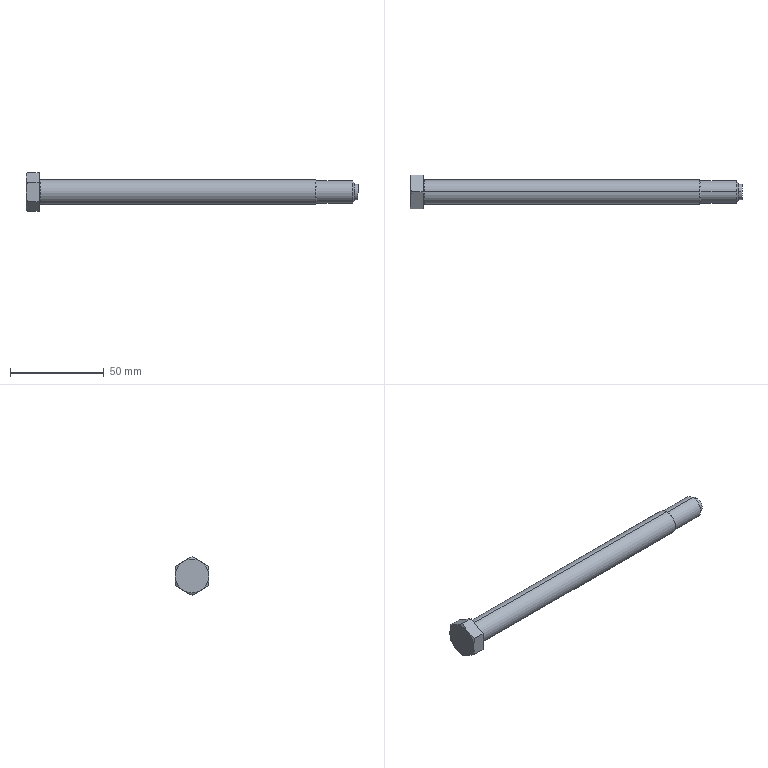Part | SolidWorks | features RevCut 2, Chamfer 1, Extrusion 1, Fillet 1, LPattern 1, MoveCopyBody 1, Revolution 1 | 1 solid | 29 faces | box 177 x 18 x 20.785 mm | volume 23953 mm3 | cone 11 | plane 10 | cylinder 6 | torus 2 | commonest cylinder face diameters 8.5 x2 12 x2 13 x2
STEP:
#1=CARTESIAN_POINT('',(-155.4,0.,169.5));
#2=VERTEX_POINT('',#1);
#3=CARTESIAN_POINT('',(-155.4,0.,156.5));
#4=VERTEX_POINT('',#3);
#5=CARTESIAN_POINT('',(-155.4,0.,163.));
#6=DIRECTION('',(1.,0.,0.));
#7=DIRECTION('',(0.,0.,-1.));
#8=AXIS2_PLACEMENT_3D('',#5,#6,#7);
#9=CIRCLE('',#8,6.5);
#10=EDGE_CURVE('',#2,#4,#9,.T.);
#11=ORIENTED_EDGE('',*,*,#10,.F.);
#12=CARTESIAN_POINT('',(-156.,0.,170.1));
#13=VERTEX_POINT('',#12);
#14=CARTESIAN_POINT('',(-155.4,0.,170.1));
#15=DIRECTION('',(0.,1.,0.));
#16=DIRECTION('',(0.,0.,1.));
#17=AXIS2_PLACEMENT_3D('',#14,#15,#16);
#18=CIRCLE('',#17,0.6);
#19=EDGE_CURVE('',#2,#13,#18,.T.);
#20=ORIENTED_EDGE('',*,*,#19,.T.);
#21=CARTESIAN_POINT('',(-156.,0.,155.9));
#22=VERTEX_POINT('',#21);
#23=CARTESIAN_POINT('',(-156.,0.,163.));
#24=DIRECTION('',(-1.,0.,0.));
#25=DIRECTION('',(0.,0.,-1.));
#26=AXIS2_PLACEMENT_3D('',#23,#24,#25);
#27=CIRCLE('',#26,7.1);
#28=EDGE_CURVE('',#22,#13,#27,.T.);
#29=ORIENTED_EDGE('',*,*,#28,.F.);
#30=CARTESIAN_POINT('',(-155.4,0.,155.9));
#31=DIRECTION('',(0.,-1.,0.));
#32=DIRECTION('',(0.,0.,-1.));
#33=AXIS2_PLACEMENT_3D('',#30,#31,#32);
#34=CIRCLE('',#33,0.6);
#35=EDGE_CURVE('',#4,#22,#34,.T.);
#36=ORIENTED_EDGE('',*,*,#35,.F.);
#37=EDGE_LOOP('',(#11,#20,#29,#36));
#38=FACE_OUTER_BOUND('',#37,.T.);
#39=CARTESIAN_POINT('',(-155.4,0.,163.));
#40=DIRECTION('',(1.,0.,0.));
#41=DIRECTION('',(0.,0.,-1.));
#42=AXIS2_PLACEMENT_3D('',#39,#40,#41);
#43=TOROIDAL_SURFACE('',#42,7.1,0.6);
#44=ADVANCED_FACE('',(#38),#43,.F.);
#45=CARTESIAN_POINT('',(-8.,0.,169.));
#46=VERTEX_POINT('',#45);
#47=CARTESIAN_POINT('',(-8.,0.,157.));
#48=VERTEX_POINT('',#47);
#49=CARTESIAN_POINT('',(-8.,0.,163.));
#50=DIRECTION('',(-1.,0.,0.));
#51=DIRECTION('',(0.,0.,1.));
#52=AXIS2_PLACEMENT_3D('',#49,#50,#51);
#53=CIRCLE('',#52,6.);
#54=EDGE_CURVE('',#46,#48,#53,.T.);
#55=ORIENTED_EDGE('',*,*,#54,.T.);
#56=CARTESIAN_POINT('',(-8.5,0.,156.5));
#57=VERTEX_POINT('',#56);
#58=CARTESIAN_POINT('',(-8.5,0.,156.5));
#59=DIRECTION('',(-0.7071,0.,-0.7071));
#60=VECTOR('',#59,1000.);
#61=LINE('',#58,#60);
#62=EDGE_CURVE('',#48,#57,#61,.T.);
#63=ORIENTED_EDGE('',*,*,#62,.T.);
#64=CARTESIAN_POINT('',(-8.5,0.,169.5));
#65=VERTEX_POINT('',#64);
#66=CARTESIAN_POINT('',(-8.5,0.,163.));
#67=DIRECTION('',(-1.,0.,0.));
#68=DIRECTION('',(0.,0.,1.));
#69=AXIS2_PLACEMENT_3D('',#66,#67,#68);
#70=CIRCLE('',#69,6.5);
#71=EDGE_CURVE('',#65,#57,#70,.T.);
#72=ORIENTED_EDGE('',*,*,#71,.F.);
#73=CARTESIAN_POINT('',(-8.5,0.,169.5));
#74=DIRECTION('',(-0.7071,0.,0.7071));
#75=VECTOR('',#74,1000.);
#76=LINE('',#73,#75);
#77=EDGE_CURVE('',#46,#65,#76,.T.);
#78=ORIENTED_EDGE('',*,*,#77,.F.);
#79=EDGE_LOOP('',(#55,#63,#72,#78));
#80=FACE_OUTER_BOUND('',#79,.T.);
#81=CARTESIAN_POINT('',(-8.5,0.,163.));
#82=DIRECTION('',(-1.,0.,0.));
#83=DIRECTION('',(0.,0.,1.));
#84=AXIS2_PLACEMENT_3D('',#81,#82,#83);
#85=CONICAL_SURFACE('',#84,6.5,0.7854);
#86=ADVANCED_FACE('',(#80),#85,.T.);
#87=CARTESIAN_POINT('',(14.,0.,167.25));
#88=VERTEX_POINT('',#87);
#89=CARTESIAN_POINT('',(14.,0.,158.75));
#90=VERTEX_POINT('',#89);
#91=CARTESIAN_POINT('',(14.,0.,163.));
#92=DIRECTION('',(-1.,0.,0.));
#93=DIRECTION('',(0.,0.,1.));
#94=AXIS2_PLACEMENT_3D('',#91,#92,#93);
#95=CIRCLE('',#94,4.25);
#96=EDGE_CURVE('',#88,#90,#95,.T.);
#97=ORIENTED_EDGE('',*,*,#96,.T.);
#98=CARTESIAN_POINT('',(12.,0.,158.75));
#99=VERTEX_POINT('',#98);
#100=CARTESIAN_POINT('',(-163.,0.,158.75));
#101=DIRECTION('',(-1.,0.,0.));
#102=VECTOR('',#101,1000.);
#103=LINE('',#100,#102);
#104=EDGE_CURVE('',#90,#99,#103,.T.);
#105=ORIENTED_EDGE('',*,*,#104,.T.);
#106=CARTESIAN_POINT('',(12.,0.,167.25));
#107=VERTEX_POINT('',#106);
#108=CARTESIAN_POINT('',(12.,0.,163.));
#109=DIRECTION('',(-1.,0.,0.));
#110=DIRECTION('',(0.,0.,1.));
#111=AXIS2_PLACEMENT_3D('',#108,#109,#110);
#112=CIRCLE('',#111,4.25);
#113=EDGE_CURVE('',#107,#99,#112,.T.);
#114=ORIENTED_EDGE('',*,*,#113,.F.);
#115=CARTESIAN_POINT('',(-163.,0.,167.25));
#116=DIRECTION('',(-1.,0.,0.));
#117=VECTOR('',#116,1000.);
#118=LINE('',#115,#117);
#119=EDGE_CURVE('',#88,#107,#118,.T.);
#120=ORIENTED_EDGE('',*,*,#119,.F.);
#121=EDGE_LOOP('',(#97,#105,#114,#120));
#122=FACE_OUTER_BOUND('',#121,.T.);
#123=CARTESIAN_POINT('',(-163.,0.,163.));
#124=DIRECTION('',(-1.,0.,0.));
#125=DIRECTION('',(0.,0.,1.));
#126=AXIS2_PLACEMENT_3D('',#123,#124,#125);
#127=CYLINDRICAL_SURFACE('',#126,4.25);
#128=ADVANCED_FACE('',(#122),#127,.T.);
#129=CARTESIAN_POINT('',(12.,0.,167.484));
#130=VERTEX_POINT('',#129);
#131=CARTESIAN_POINT('',(12.,0.,158.516));
#132=VERTEX_POINT('',#131);
#133=CARTESIAN_POINT('',(12.,0.,163.));
#134=DIRECTION('',(-1.,0.,0.));
#135=DIRECTION('',(0.,0.,1.));
#136=AXIS2_PLACEMENT_3D('',#133,#134,#135);
#137=CIRCLE('',#136,4.484);
#138=EDGE_CURVE('',#130,#132,#137,.T.);
#139=ORIENTED_EDGE('',*,*,#138,.T.);
#140=CARTESIAN_POINT('',(11.125,0.,157.));
#141=VERTEX_POINT('',#140);
#142=CARTESIAN_POINT('',(11.125,0.,157.));
#143=DIRECTION('',(-0.5,0.,-0.866));
#144=VECTOR('',#143,1000.);
#145=LINE('',#142,#144);
#146=EDGE_CURVE('',#132,#141,#145,.T.);
#147=ORIENTED_EDGE('',*,*,#146,.T.);
#148=CARTESIAN_POINT('',(11.125,0.,169.));
#149=VERTEX_POINT('',#148);
#150=CARTESIAN_POINT('',(11.125,0.,163.));
#151=DIRECTION('',(-1.,0.,0.));
#152=DIRECTION('',(0.,0.,1.));
#153=AXIS2_PLACEMENT_3D('',#150,#151,#152);
#154=CIRCLE('',#153,6.);
#155=EDGE_CURVE('',#149,#141,#154,.T.);
#156=ORIENTED_EDGE('',*,*,#155,.F.);
#157=CARTESIAN_POINT('',(11.125,0.,169.));
#158=DIRECTION('',(-0.5,0.,0.866));
#159=VECTOR('',#158,1000.);
#160=LINE('',#157,#159);
#161=EDGE_CURVE('',#130,#149,#160,.T.);
#162=ORIENTED_EDGE('',*,*,#161,.F.);
#163=EDGE_LOOP('',(#139,#147,#156,#162));
#164=FACE_OUTER_BOUND('',#163,.T.);
#165=CARTESIAN_POINT('',(11.125,0.,163.));
#166=DIRECTION('',(-1.,0.,0.));
#167=DIRECTION('',(0.,0.,1.));
#168=AXIS2_PLACEMENT_3D('',#165,#166,#167);
#169=CONICAL_SURFACE('',#168,6.,1.047);
#170=ADVANCED_FACE('',(#164),#169,.T.);
#171=ORIENTED_EDGE('',*,*,#71,.T.);
#172=CARTESIAN_POINT('',(-163.,0.,156.5));
#173=DIRECTION('',(-1.,0.,0.));
#174=VECTOR('',#173,1000.);
#175=LINE('',#172,#174);
#176=EDGE_CURVE('',#57,#4,#175,.T.);
#177=ORIENTED_EDGE('',*,*,#176,.T.);
#178=CARTESIAN_POINT('',(-155.4,0.,163.));
#179=DIRECTION('',(1.,0.,0.));
#180=DIRECTION('',(0.,0.,-1.));
#181=AXIS2_PLACEMENT_3D('',#178,#179,#180);
#182=CIRCLE('',#181,6.5);
#183=EDGE_CURVE('',#4,#2,#182,.T.);
#184=ORIENTED_EDGE('',*,*,#183,.T.);
#185=CARTESIAN_POINT('',(-163.,0.,169.5));
#186=DIRECTION('',(-1.,0.,0.));
#187=VECTOR('',#186,1000.);
#188=LINE('',#185,#187);
#189=EDGE_CURVE('',#65,#2,#188,.T.);
#190=ORIENTED_EDGE('',*,*,#189,.F.);
#191=EDGE_LOOP('',(#171,#177,#184,#190));
#192=FACE_OUTER_BOUND('',#191,.T.);
#193=CARTESIAN_POINT('',(-163.,0.,163.));
#194=DIRECTION('',(-1.,0.,0.));
#195=DIRECTION('',(0.,0.,1.));
#196=AXIS2_PLACEMENT_3D('',#193,#194,#195);
#197=CYLINDRICAL_SURFACE('',#196,6.5);
#198=ADVANCED_FACE('',(#192),#197,.T.);
#199=CARTESIAN_POINT('',(-163.,0.,154.));
#200=VERTEX_POINT('',#199);
#201=CARTESIAN_POINT('',(-163.,-4.5,155.206));
#202=VERTEX_POINT('',#201);
#203=CARTESIAN_POINT('',(-163.,0.,163.));
#204=DIRECTION('',(-1.,0.,0.));
#205=DIRECTION('',(0.,0.,-1.));
#206=AXIS2_PLACEMENT_3D('',#203,#204,#205);
#207=CIRCLE('',#206,9.);
#208=EDGE_CURVE('',#200,#202,#207,.T.);
#209=ORIENTED_EDGE('',*,*,#208,.F.);
#210=CARTESIAN_POINT('',(-162.196,0.,152.608));
#211=VERTEX_POINT('',#210);
#212=CARTESIAN_POINT('',(-162.196,0.,152.608));
#213=DIRECTION('',(0.5,0.,-0.866));
#214=VECTOR('',#213,1000.);
#215=LINE('',#212,#214);
#216=EDGE_CURVE('',#200,#211,#215,.T.);
#217=ORIENTED_EDGE('',*,*,#216,.T.);
#218=CARTESIAN_POINT('',(-163.,-4.5,155.206));
#219=CARTESIAN_POINT('',(-163.,-4.118,154.985));
#220=CARTESIAN_POINT('',(-162.981,-3.734,154.764));
#221=CARTESIAN_POINT('',(-162.907,-2.976,154.326));
#222=CARTESIAN_POINT('',(-162.853,-2.599,154.108));
#223=CARTESIAN_POINT('',(-162.643,-1.475,153.459));
#224=CARTESIAN_POINT('',(-162.441,-0.7343,153.032));
#225=CARTESIAN_POINT('',(-162.196,0.,152.608));
#226=B_SPLINE_CURVE_WITH_KNOTS('',3,(#218,#219,#220,#221,#222,#223,#224,#225),.UNSPECIFIED.,.F.,.F.,(4,2,2,4),(0.005258,0.006567,0.007877,0.0105),.UNSPECIFIED.);
#227=EDGE_CURVE('',#202,#211,#226,.T.);
#228=ORIENTED_EDGE('',*,*,#227,.F.);
#229=EDGE_LOOP('',(#209,#217,#228));
#230=FACE_OUTER_BOUND('',#229,.T.);
#231=CARTESIAN_POINT('',(-162.196,0.,163.));
#232=DIRECTION('',(1.,0.,0.));
#233=DIRECTION('',(0.,0.,-1.));
#234=AXIS2_PLACEMENT_3D('',#231,#232,#233);
#235=CONICAL_SURFACE('',#234,10.392,1.047);
#236=ADVANCED_FACE('',(#230),#235,.T.);
#237=ORIENTED_EDGE('',*,*,#155,.T.);
#238=CARTESIAN_POINT('',(-163.,0.,157.));
#239=DIRECTION('',(-1.,0.,0.));
#240=VECTOR('',#239,1000.);
#241=LINE('',#238,#240);
#242=EDGE_CURVE('',#141,#48,#241,.T.);
#243=ORIENTED_EDGE('',*,*,#242,.T.);
#244=ORIENTED_EDGE('',*,*,#54,.F.);
#245=CARTESIAN_POINT('',(-163.,0.,169.));
#246=DIRECTION('',(-1.,0.,0.));
#247=VECTOR('',#246,1000.);
#248=LINE('',#245,#247);
#249=EDGE_CURVE('',#149,#46,#248,.T.);
#250=ORIENTED_EDGE('',*,*,#249,.F.);
#251=EDGE_LOOP('',(#237,#243,#244,#250));
#252=FACE_OUTER_BOUND('',#251,.T.);
#253=CARTESIAN_POINT('',(-163.,0.,163.));
#254=DIRECTION('',(-1.,0.,0.));
#255=DIRECTION('',(0.,0.,1.));
#256=AXIS2_PLACEMENT_3D('',#253,#254,#255);
#257=CYLINDRICAL_SURFACE('',#256,6.);
#258=ADVANCED_FACE('',(#252),#257,.T.);
#259=ORIENTED_EDGE('',*,*,#242,.F.);
#260=CARTESIAN_POINT('',(11.125,0.,163.));
#261=DIRECTION('',(-1.,0.,0.));
#262=DIRECTION('',(0.,0.,1.));
#263=AXIS2_PLACEMENT_3D('',#260,#261,#262);
#264=CIRCLE('',#263,6.);
#265=EDGE_CURVE('',#141,#149,#264,.T.);
#266=ORIENTED_EDGE('',*,*,#265,.T.);
#267=ORIENTED_EDGE('',*,*,#249,.T.);
#268=CARTESIAN_POINT('',(-8.,0.,163.));
#269=DIRECTION('',(-1.,0.,0.));
#270=DIRECTION('',(0.,0.,1.));
#271=AXIS2_PLACEMENT_3D('',#268,#269,#270);
#272=CIRCLE('',#271,6.);
#273=EDGE_CURVE('',#48,#46,#272,.T.);
#274=ORIENTED_EDGE('',*,*,#273,.F.);
#275=EDGE_LOOP('',(#259,#266,#267,#274));
#276=FACE_OUTER_BOUND('',#275,.T.);
#277=CARTESIAN_POINT('',(-163.,0.,163.));
#278=DIRECTION('',(-1.,0.,0.));
#279=DIRECTION('',(0.,0.,1.));
#280=AXIS2_PLACEMENT_3D('',#277,#278,#279);
#281=CYLINDRICAL_SURFACE('',#280,6.);
#282=ADVANCED_FACE('',(#276),#281,.T.);
#283=ORIENTED_EDGE('',*,*,#28,.T.);
#284=CARTESIAN_POINT('',(-156.,0.,163.));
#285=DIRECTION('',(-1.,0.,0.));
#286=DIRECTION('',(0.,0.,-1.));
#287=AXIS2_PLACEMENT_3D('',#284,#285,#286);
#288=CIRCLE('',#287,7.1);
#289=EDGE_CURVE('',#13,#22,#288,.T.);
#290=ORIENTED_EDGE('',*,*,#289,.T.);
#291=EDGE_LOOP('',(#283,#290));
#292=FACE_BOUND('',#291,.T.);
#293=CARTESIAN_POINT('',(-156.,-9.,157.804));
#294=VERTEX_POINT('',#293);
#295=CARTESIAN_POINT('',(-156.,0.,152.608));
#296=VERTEX_POINT('',#295);
#297=CARTESIAN_POINT('',(-156.,-9.,157.804));
#298=DIRECTION('',(0.,0.866,-0.5));
#299=VECTOR('',#298,1000.);
#300=LINE('',#297,#299);
#301=EDGE_CURVE('',#294,#296,#300,.T.);
#302=ORIENTED_EDGE('',*,*,#301,.T.);
#303=CARTESIAN_POINT('',(-156.,9.,157.804));
#304=VERTEX_POINT('',#303);
#305=CARTESIAN_POINT('',(-156.,0.,152.608));
#306=DIRECTION('',(0.,0.866,0.5));
#307=VECTOR('',#306,1000.);
#308=LINE('',#305,#307);
#309=EDGE_CURVE('',#296,#304,#308,.T.);
#310=ORIENTED_EDGE('',*,*,#309,.T.);
#311=CARTESIAN_POINT('',(-156.,9.,168.196));
#312=VERTEX_POINT('',#311);
#313=CARTESIAN_POINT('',(-156.,9.,157.804));
#314=DIRECTION('',(0.,0.,1.));
#315=VECTOR('',#314,1000.);
#316=LINE('',#313,#315);
#317=EDGE_CURVE('',#304,#312,#316,.T.);
#318=ORIENTED_EDGE('',*,*,#317,.T.);
#319=CARTESIAN_POINT('',(-156.,0.,173.392));
#320=VERTEX_POINT('',#319);
#321=CARTESIAN_POINT('',(-156.,9.,168.196));
#322=DIRECTION('',(0.,-0.866,0.5));
#323=VECTOR('',#322,1000.);
#324=LINE('',#321,#323);
#325=EDGE_CURVE('',#312,#320,#324,.T.);
#326=ORIENTED_EDGE('',*,*,#325,.T.);
#327=CARTESIAN_POINT('',(-156.,-9.,168.196));
#328=VERTEX_POINT('',#327);
#329=CARTESIAN_POINT('',(-156.,0.,173.392));
#330=DIRECTION('',(0.,-0.866,-0.5));
#331=VECTOR('',#330,1000.);
#332=LINE('',#329,#331);
#333=EDGE_CURVE('',#320,#328,#332,.T.);
#334=ORIENTED_EDGE('',*,*,#333,.T.);
#335=CARTESIAN_POINT('',(-156.,-9.,168.196));
#336=DIRECTION('',(0.,0.,-1.));
#337=VECTOR('',#336,1000.);
#338=LINE('',#335,#337);
#339=EDGE_CURVE('',#328,#294,#338,.T.);
#340=ORIENTED_EDGE('',*,*,#339,.T.);
#341=EDGE_LOOP('',(#302,#310,#318,#326,#334,#340));
#342=FACE_OUTER_BOUND('',#341,.T.);
#343=CARTESIAN_POINT('',(-156.,0.,152.608));
#344=DIRECTION('',(1.,0.,0.));
#345=DIRECTION('',(0.,0.,-1.));
#346=AXIS2_PLACEMENT_3D('',#343,#344,#345);
#347=PLANE('',#346);
#348=ADVANCED_FACE('',(#292,#342),#347,.T.);
#349=CARTESIAN_POINT('',(-162.196,-9.,157.804));
#350=VERTEX_POINT('',#349);
#351=CARTESIAN_POINT('',(-156.,-9.,157.804));
#352=DIRECTION('',(-1.,0.,0.));
#353=VECTOR('',#352,1000.);
#354=LINE('',#351,#353);
#355=EDGE_CURVE('',#294,#350,#354,.T.);
#356=ORIENTED_EDGE('',*,*,#355,.T.);
#357=CARTESIAN_POINT('',(-162.196,-9.,157.804));
#358=CARTESIAN_POINT('',(-162.442,-8.264,157.379));
#359=CARTESIAN_POINT('',(-162.644,-7.522,156.951));
#360=CARTESIAN_POINT('',(-162.923,-6.024,156.086));
#361=CARTESIAN_POINT('',(-163.,-5.267,155.648));
#362=CARTESIAN_POINT('',(-163.,-4.5,155.206));
#363=B_SPLINE_CURVE_WITH_KNOTS('',3,(#357,#358,#359,#360,#361,#362),.UNSPECIFIED.,.F.,.F.,(4,2,4),(0.000000238,0.002629,0.005258),.UNSPECIFIED.);
#364=EDGE_CURVE('',#350,#202,#363,.T.);
#365=ORIENTED_EDGE('',*,*,#364,.T.);
#366=ORIENTED_EDGE('',*,*,#227,.T.);
#367=CARTESIAN_POINT('',(-156.,0.,152.608));
#368=DIRECTION('',(-1.,0.,0.));
#369=VECTOR('',#368,1000.);
#370=LINE('',#367,#369);
#371=EDGE_CURVE('',#296,#211,#370,.T.);
#372=ORIENTED_EDGE('',*,*,#371,.F.);
#373=ORIENTED_EDGE('',*,*,#301,.F.);
#374=EDGE_LOOP('',(#356,#365,#366,#372,#373));
#375=FACE_OUTER_BOUND('',#374,.T.);
#376=CARTESIAN_POINT('',(-156.,-9.,157.804));
#377=DIRECTION('',(0.,0.5,0.866));
#378=DIRECTION('',(0.,-0.866,0.5));
#379=AXIS2_PLACEMENT_3D('',#376,#377,#378);
#380=PLANE('',#379);
#381=ADVANCED_FACE('',(#375),#380,.F.);
#382=ORIENTED_EDGE('',*,*,#371,.T.);
#383=CARTESIAN_POINT('',(-163.,4.5,155.206));
#384=VERTEX_POINT('',#383);
#385=CARTESIAN_POINT('',(-162.196,0.,152.608));
#386=CARTESIAN_POINT('',(-162.442,0.7361,153.033));
#387=CARTESIAN_POINT('',(-162.644,1.478,153.461));
#388=CARTESIAN_POINT('',(-162.923,2.976,154.326));
#389=CARTESIAN_POINT('',(-163.,3.733,154.763));
#390=CARTESIAN_POINT('',(-163.,4.5,155.206));
#391=B_SPLINE_CURVE_WITH_KNOTS('',3,(#385,#386,#387,#388,#389,#390),.UNSPECIFIED.,.F.,.F.,(4,2,4),(0.000000238,0.002629,0.005258),.UNSPECIFIED.);
#392=EDGE_CURVE('',#211,#384,#391,.T.);
#393=ORIENTED_EDGE('',*,*,#392,.T.);
#394=CARTESIAN_POINT('',(-162.196,9.,157.804));
#395=VERTEX_POINT('',#394);
#396=CARTESIAN_POINT('',(-163.,4.5,155.206));
#397=CARTESIAN_POINT('',(-163.,4.882,155.426));
#398=CARTESIAN_POINT('',(-162.981,5.266,155.648));
#399=CARTESIAN_POINT('',(-162.907,6.024,156.086));
#400=CARTESIAN_POINT('',(-162.853,6.401,156.303));
#401=CARTESIAN_POINT('',(-162.643,7.525,156.952));
#402=CARTESIAN_POINT('',(-162.441,8.266,157.38));
#403=CARTESIAN_POINT('',(-162.196,9.,157.804));
#404=B_SPLINE_CURVE_WITH_KNOTS('',3,(#396,#397,#398,#399,#400,#401,#402,#403),.UNSPECIFIED.,.F.,.F.,(4,2,2,4),(0.005258,0.006567,0.007877,0.0105),.UNSPECIFIED.);
#405=EDGE_CURVE('',#384,#395,#404,.T.);
#406=ORIENTED_EDGE('',*,*,#405,.T.);
#407=CARTESIAN_POINT('',(-156.,9.,157.804));
#408=DIRECTION('',(-1.,0.,0.));
#409=VECTOR('',#408,1000.);
#410=LINE('',#407,#409);
#411=EDGE_CURVE('',#304,#395,#410,.T.);
#412=ORIENTED_EDGE('',*,*,#411,.F.);
#413=ORIENTED_EDGE('',*,*,#309,.F.);
#414=EDGE_LOOP('',(#382,#393,#406,#412,#413));
#415=FACE_OUTER_BOUND('',#414,.T.);
#416=CARTESIAN_POINT('',(-156.,0.,152.608));
#417=DIRECTION('',(0.,-0.5,0.866));
#418=DIRECTION('',(0.,-0.866,-0.5));
#419=AXIS2_PLACEMENT_3D('',#416,#417,#418);
#420=PLANE('',#419);
#421=ADVANCED_FACE('',(#415),#420,.F.);
#422=ORIENTED_EDGE('',*,*,#411,.T.);
#423=CARTESIAN_POINT('',(-163.,9.,163.));
#424=VERTEX_POINT('',#423);
#425=CARTESIAN_POINT('',(-162.196,9.,157.804));
#426=CARTESIAN_POINT('',(-162.439,9.,158.644));
#427=CARTESIAN_POINT('',(-162.641,9.,159.495));
#428=CARTESIAN_POINT('',(-162.922,9.,161.231));
#429=CARTESIAN_POINT('',(-163.,9.,162.121));
#430=CARTESIAN_POINT('',(-163.,9.,163.));
#431=B_SPLINE_CURVE_WITH_KNOTS('',3,(#425,#426,#427,#428,#429,#430),.UNSPECIFIED.,.F.,.F.,(4,2,4),(0.003809,0.006432,0.009055),.UNSPECIFIED.);
#432=EDGE_CURVE('',#395,#424,#431,.T.);
#433=ORIENTED_EDGE('',*,*,#432,.T.);
#434=CARTESIAN_POINT('',(-162.196,9.,168.196));
#435=VERTEX_POINT('',#434);
#436=CARTESIAN_POINT('',(-163.,9.,163.));
#437=CARTESIAN_POINT('',(-163.,9.,163.878));
#438=CARTESIAN_POINT('',(-162.925,9.,164.75));
#439=CARTESIAN_POINT('',(-162.645,9.,166.485));
#440=CARTESIAN_POINT('',(-162.44,9.,167.351));
#441=CARTESIAN_POINT('',(-162.196,9.,168.196));
#442=B_SPLINE_CURVE_WITH_KNOTS('',3,(#436,#437,#438,#439,#440,#441),.UNSPECIFIED.,.F.,.F.,(4,2,4),(0.009055,0.01168,0.0143),.UNSPECIFIED.);
#443=EDGE_CURVE('',#424,#435,#442,.T.);
#444=ORIENTED_EDGE('',*,*,#443,.T.);
#445=CARTESIAN_POINT('',(-156.,9.,168.196));
#446=DIRECTION('',(-1.,0.,0.));
#447=VECTOR('',#446,1000.);
#448=LINE('',#445,#447);
#449=EDGE_CURVE('',#312,#435,#448,.T.);
#450=ORIENTED_EDGE('',*,*,#449,.F.);
#451=ORIENTED_EDGE('',*,*,#317,.F.);
#452=EDGE_LOOP('',(#422,#433,#444,#450,#451));
#453=FACE_OUTER_BOUND('',#452,.T.);
#454=CARTESIAN_POINT('',(-156.,9.,157.804));
#455=DIRECTION('',(0.,-1.,0.));
#456=DIRECTION('',(-1.,0.,0.));
#457=AXIS2_PLACEMENT_3D('',#454,#455,#456);
#458=PLANE('',#457);
#459=ADVANCED_FACE('',(#453),#458,.F.);
#460=ORIENTED_EDGE('',*,*,#449,.T.);
#461=CARTESIAN_POINT('',(-163.,4.5,170.794));
#462=VERTEX_POINT('',#461);
#463=CARTESIAN_POINT('',(-162.196,9.,168.196));
#464=CARTESIAN_POINT('',(-162.442,8.264,168.621));
#465=CARTESIAN_POINT('',(-162.644,7.522,169.049));
#466=CARTESIAN_POINT('',(-162.923,6.024,169.914));
#467=CARTESIAN_POINT('',(-163.,5.267,170.352));
#468=CARTESIAN_POINT('',(-163.,4.5,170.794));
#469=B_SPLINE_CURVE_WITH_KNOTS('',3,(#463,#464,#465,#466,#467,#468),.UNSPECIFIED.,.F.,.F.,(4,2,4),(0.000000238,0.002629,0.005258),.UNSPECIFIED.);
#470=EDGE_CURVE('',#435,#462,#469,.T.);
#471=ORIENTED_EDGE('',*,*,#470,.T.);
#472=CARTESIAN_POINT('',(-162.196,0.,173.392));
#473=VERTEX_POINT('',#472);
#474=CARTESIAN_POINT('',(-163.,4.5,170.794));
#475=CARTESIAN_POINT('',(-163.,4.118,171.015));
#476=CARTESIAN_POINT('',(-162.981,3.734,171.236));
#477=CARTESIAN_POINT('',(-162.907,2.976,171.674));
#478=CARTESIAN_POINT('',(-162.853,2.599,171.892));
#479=CARTESIAN_POINT('',(-162.643,1.475,172.541));
#480=CARTESIAN_POINT('',(-162.441,0.7343,172.968));
#481=CARTESIAN_POINT('',(-162.196,0.,173.392));
#482=B_SPLINE_CURVE_WITH_KNOTS('',3,(#474,#475,#476,#477,#478,#479,#480,#481),.UNSPECIFIED.,.F.,.F.,(4,2,2,4),(0.005258,0.006567,0.007877,0.0105),.UNSPECIFIED.);
#483=EDGE_CURVE('',#462,#473,#482,.T.);
#484=ORIENTED_EDGE('',*,*,#483,.T.);
#485=CARTESIAN_POINT('',(-156.,0.,173.392));
#486=DIRECTION('',(-1.,0.,0.));
#487=VECTOR('',#486,1000.);
#488=LINE('',#485,#487);
#489=EDGE_CURVE('',#320,#473,#488,.T.);
#490=ORIENTED_EDGE('',*,*,#489,.F.);
#491=ORIENTED_EDGE('',*,*,#325,.F.);
#492=EDGE_LOOP('',(#460,#471,#484,#490,#491));
#493=FACE_OUTER_BOUND('',#492,.T.);
#494=CARTESIAN_POINT('',(-156.,9.,168.196));
#495=DIRECTION('',(0.,-0.5,-0.866));
#496=DIRECTION('',(0.,0.866,-0.5));
#497=AXIS2_PLACEMENT_3D('',#494,#495,#496);
#498=PLANE('',#497);
#499=ADVANCED_FACE('',(#493),#498,.F.);
#500=ORIENTED_EDGE('',*,*,#489,.T.);
#501=CARTESIAN_POINT('',(-163.,-4.5,170.794));
#502=VERTEX_POINT('',#501);
#503=CARTESIAN_POINT('',(-162.196,0.,173.392));
#504=CARTESIAN_POINT('',(-162.442,-0.7361,172.967));
#505=CARTESIAN_POINT('',(-162.644,-1.478,172.539));
#506=CARTESIAN_POINT('',(-162.923,-2.976,171.674));
#507=CARTESIAN_POINT('',(-163.,-3.733,171.237));
#508=CARTESIAN_POINT('',(-163.,-4.5,170.794));
#509=B_SPLINE_CURVE_WITH_KNOTS('',3,(#503,#504,#505,#506,#507,#508),.UNSPECIFIED.,.F.,.F.,(4,2,4),(0.000000238,0.002629,0.005258),.UNSPECIFIED.);
#510=EDGE_CURVE('',#473,#502,#509,.T.);
#511=ORIENTED_EDGE('',*,*,#510,.T.);
#512=CARTESIAN_POINT('',(-162.196,-9.,168.196));
#513=VERTEX_POINT('',#512);
#514=CARTESIAN_POINT('',(-163.,-4.5,170.794));
#515=CARTESIAN_POINT('',(-163.,-4.882,170.574));
#516=CARTESIAN_POINT('',(-162.981,-5.266,170.352));
#517=CARTESIAN_POINT('',(-162.907,-6.024,169.914));
#518=CARTESIAN_POINT('',(-162.853,-6.401,169.697));
#519=CARTESIAN_POINT('',(-162.643,-7.525,169.048));
#520=CARTESIAN_POINT('',(-162.441,-8.266,168.62));
#521=CARTESIAN_POINT('',(-162.196,-9.,168.196));
#522=B_SPLINE_CURVE_WITH_KNOTS('',3,(#514,#515,#516,#517,#518,#519,#520,#521),.UNSPECIFIED.,.F.,.F.,(4,2,2,4),(0.005258,0.006567,0.007877,0.0105),.UNSPECIFIED.);
#523=EDGE_CURVE('',#502,#513,#522,.T.);
#524=ORIENTED_EDGE('',*,*,#523,.T.);
#525=CARTESIAN_POINT('',(-156.,-9.,168.196));
#526=DIRECTION('',(-1.,0.,0.));
#527=VECTOR('',#526,1000.);
#528=LINE('',#525,#527);
#529=EDGE_CURVE('',#328,#513,#528,.T.);
#530=ORIENTED_EDGE('',*,*,#529,.F.);
#531=ORIENTED_EDGE('',*,*,#333,.F.);
#532=EDGE_LOOP('',(#500,#511,#524,#530,#531));
#533=FACE_OUTER_BOUND('',#532,.T.);
#534=CARTESIAN_POINT('',(-156.,0.,173.392));
#535=DIRECTION('',(0.,0.5,-0.866));
#536=DIRECTION('',(0.,0.866,0.5));
#537=AXIS2_PLACEMENT_3D('',#534,#535,#536);
#538=PLANE('',#537);
#539=ADVANCED_FACE('',(#533),#538,.F.);
#540=ORIENTED_EDGE('',*,*,#529,.T.);
#541=CARTESIAN_POINT('',(-163.,-9.,163.));
#542=VERTEX_POINT('',#541);
#543=CARTESIAN_POINT('',(-162.196,-9.,168.196));
#544=CARTESIAN_POINT('',(-162.44,-9.,167.351));
#545=CARTESIAN_POINT('',(-162.645,-9.,166.485));
#546=CARTESIAN_POINT('',(-162.925,-9.,164.75));
#547=CARTESIAN_POINT('',(-163.,-9.,163.878));
#548=CARTESIAN_POINT('',(-163.,-9.,163.));
#549=B_SPLINE_CURVE_WITH_KNOTS('',3,(#543,#544,#545,#546,#547,#548),.UNSPECIFIED.,.F.,.F.,(4,2,4),(0.009271,0.0119,0.01453),.UNSPECIFIED.);
#550=EDGE_CURVE('',#513,#542,#549,.T.);
#551=ORIENTED_EDGE('',*,*,#550,.T.);
#552=CARTESIAN_POINT('',(-163.,-9.,163.));
#553=CARTESIAN_POINT('',(-163.,-9.,162.121));
#554=CARTESIAN_POINT('',(-162.922,-9.,161.231));
#555=CARTESIAN_POINT('',(-162.641,-9.,159.495));
#556=CARTESIAN_POINT('',(-162.439,-9.,158.644));
#557=CARTESIAN_POINT('',(-162.196,-9.,157.804));
#558=B_SPLINE_CURVE_WITH_KNOTS('',3,(#552,#553,#554,#555,#556,#557),.UNSPECIFIED.,.F.,.F.,(4,2,4),(0.01453,0.01716,0.01979),.UNSPECIFIED.);
#559=EDGE_CURVE('',#542,#350,#558,.T.);
#560=ORIENTED_EDGE('',*,*,#559,.T.);
#561=ORIENTED_EDGE('',*,*,#355,.F.);
#562=ORIENTED_EDGE('',*,*,#339,.F.);
#563=EDGE_LOOP('',(#540,#551,#560,#561,#562));
#564=FACE_OUTER_BOUND('',#563,.T.);
#565=CARTESIAN_POINT('',(-156.,-9.,168.196));
#566=DIRECTION('',(0.,1.,0.));
#567=DIRECTION('',(1.,0.,0.));
#568=AXIS2_PLACEMENT_3D('',#565,#566,#567);
#569=PLANE('',#568);
#570=ADVANCED_FACE('',(#564),#569,.F.);
#571=ORIENTED_EDGE('',*,*,#216,.F.);
#572=CARTESIAN_POINT('',(-163.,0.,163.));
#573=DIRECTION('',(-1.,0.,0.));
#574=DIRECTION('',(0.,0.,-1.));
#575=AXIS2_PLACEMENT_3D('',#572,#573,#574);
#576=CIRCLE('',#575,9.);
#577=EDGE_CURVE('',#384,#200,#576,.T.);
#578=ORIENTED_EDGE('',*,*,#577,.F.);
#579=ORIENTED_EDGE('',*,*,#392,.F.);
#580=EDGE_LOOP('',(#571,#578,#579));
#581=FACE_OUTER_BOUND('',#580,.T.);
#582=CARTESIAN_POINT('',(-162.196,0.,163.));
#583=DIRECTION('',(1.,0.,0.));
#584=DIRECTION('',(0.,0.,-1.));
#585=AXIS2_PLACEMENT_3D('',#582,#583,#584);
#586=CONICAL_SURFACE('',#585,10.392,1.047);
#587=ADVANCED_FACE('',(#581),#586,.T.);
#588=CARTESIAN_POINT('',(-163.,0.,163.));
#589=DIRECTION('',(-1.,0.,0.));
#590=DIRECTION('',(0.,0.,-1.));
#591=AXIS2_PLACEMENT_3D('',#588,#589,#590);
#592=CIRCLE('',#591,9.);
#593=EDGE_CURVE('',#424,#384,#592,.T.);
#594=ORIENTED_EDGE('',*,*,#593,.F.);
#595=ORIENTED_EDGE('',*,*,#432,.F.);
#596=ORIENTED_EDGE('',*,*,#405,.F.);
#597=EDGE_LOOP('',(#594,#595,#596));
#598=FACE_OUTER_BOUND('',#597,.T.);
#599=CARTESIAN_POINT('',(-162.196,0.,163.));
#600=DIRECTION('',(1.,0.,0.));
#601=DIRECTION('',(0.,0.,-1.));
#602=AXIS2_PLACEMENT_3D('',#599,#600,#601);
#603=CONICAL_SURFACE('',#602,10.392,1.047);
#604=ADVANCED_FACE('',(#598),#603,.T.);
#605=CARTESIAN_POINT('',(-163.,0.,163.));
#606=DIRECTION('',(-1.,0.,0.));
#607=DIRECTION('',(0.,0.,1.));
#608=AXIS2_PLACEMENT_3D('',#605,#606,#607);
#609=CIRCLE('',#608,9.);
#610=EDGE_CURVE('',#462,#424,#609,.T.);
#611=ORIENTED_EDGE('',*,*,#610,.F.);
#612=ORIENTED_EDGE('',*,*,#470,.F.);
#613=ORIENTED_EDGE('',*,*,#443,.F.);
#614=EDGE_LOOP('',(#611,#612,#613));
#615=FACE_OUTER_BOUND('',#614,.T.);
#616=CARTESIAN_POINT('',(-162.196,0.,163.));
#617=DIRECTION('',(1.,0.,0.));
#618=DIRECTION('',(0.,0.,-1.));
#619=AXIS2_PLACEMENT_3D('',#616,#617,#618);
#620=CONICAL_SURFACE('',#619,10.392,1.047);
#621=ADVANCED_FACE('',(#615),#620,.T.);
#622=CARTESIAN_POINT('',(-163.,0.,163.));
#623=DIRECTION('',(-1.,0.,0.));
#624=DIRECTION('',(0.,0.,-1.));
#625=AXIS2_PLACEMENT_3D('',#622,#623,#624);
#626=CIRCLE('',#625,9.);
#627=EDGE_CURVE('',#502,#462,#626,.T.);
#628=ORIENTED_EDGE('',*,*,#627,.F.);
#629=ORIENTED_EDGE('',*,*,#510,.F.);
#630=ORIENTED_EDGE('',*,*,#483,.F.);
#631=EDGE_LOOP('',(#628,#629,#630));
#632=FACE_OUTER_BOUND('',#631,.T.);
#633=CARTESIAN_POINT('',(-162.196,0.,163.));
#634=DIRECTION('',(1.,0.,0.));
#635=DIRECTION('',(0.,0.,-1.));
#636=AXIS2_PLACEMENT_3D('',#633,#634,#635);
#637=CONICAL_SURFACE('',#636,10.392,1.047);
#638=ADVANCED_FACE('',(#632),#637,.T.);
#639=CARTESIAN_POINT('',(-163.,0.,163.));
#640=DIRECTION('',(-1.,0.,0.));
#641=DIRECTION('',(0.,0.,-1.));
#642=AXIS2_PLACEMENT_3D('',#639,#640,#641);
#643=CIRCLE('',#642,9.);
#644=EDGE_CURVE('',#542,#502,#643,.T.);
#645=ORIENTED_EDGE('',*,*,#644,.F.);
#646=ORIENTED_EDGE('',*,*,#550,.F.);
#647=ORIENTED_EDGE('',*,*,#523,.F.);
#648=EDGE_LOOP('',(#645,#646,#647));
#649=FACE_OUTER_BOUND('',#648,.T.);
#650=CARTESIAN_POINT('',(-162.196,0.,163.));
#651=DIRECTION('',(1.,0.,0.));
#652=DIRECTION('',(0.,0.,-1.));
#653=AXIS2_PLACEMENT_3D('',#650,#651,#652);
#654=CONICAL_SURFACE('',#653,10.392,1.047);
#655=ADVANCED_FACE('',(#649),#654,.T.);
#656=ORIENTED_EDGE('',*,*,#559,.F.);
#657=CARTESIAN_POINT('',(-163.,0.,163.));
#658=DIRECTION('',(-1.,0.,0.));
#659=DIRECTION('',(0.,0.,-1.));
#660=AXIS2_PLACEMENT_3D('',#657,#658,#659);
#661=CIRCLE('',#660,9.);
#662=EDGE_CURVE('',#202,#542,#661,.T.);
#663=ORIENTED_EDGE('',*,*,#662,.F.);
#664=ORIENTED_EDGE('',*,*,#364,.F.);
#665=EDGE_LOOP('',(#656,#663,#664));
#666=FACE_OUTER_BOUND('',#665,.T.);
#667=CARTESIAN_POINT('',(-162.196,0.,163.));
#668=DIRECTION('',(1.,0.,0.));
#669=DIRECTION('',(0.,0.,-1.));
#670=AXIS2_PLACEMENT_3D('',#667,#668,#669);
#671=CONICAL_SURFACE('',#670,10.392,1.047);
#672=ADVANCED_FACE('',(#666),#671,.T.);
#673=ORIENTED_EDGE('',*,*,#577,.T.);
#674=ORIENTED_EDGE('',*,*,#208,.T.);
#675=ORIENTED_EDGE('',*,*,#662,.T.);
#676=ORIENTED_EDGE('',*,*,#644,.T.);
#677=ORIENTED_EDGE('',*,*,#627,.T.);
#678=ORIENTED_EDGE('',*,*,#610,.T.);
#679=ORIENTED_EDGE('',*,*,#593,.T.);
#680=EDGE_LOOP('',(#673,#674,#675,#676,#677,#678,#679));
#681=FACE_OUTER_BOUND('',#680,.T.);
#682=CARTESIAN_POINT('',(-163.,0.,152.608));
#683=DIRECTION('',(1.,0.,0.));
#684=DIRECTION('',(0.,0.,-1.));
#685=AXIS2_PLACEMENT_3D('',#682,#683,#684);
#686=PLANE('',#685);
#687=ADVANCED_FACE('',(#681),#686,.F.);
#688=ORIENTED_EDGE('',*,*,#176,.F.);
#689=CARTESIAN_POINT('',(-8.5,0.,163.));
#690=DIRECTION('',(-1.,0.,0.));
#691=DIRECTION('',(0.,0.,1.));
#692=AXIS2_PLACEMENT_3D('',#689,#690,#691);
#693=CIRCLE('',#692,6.5);
#694=EDGE_CURVE('',#57,#65,#693,.T.);
#695=ORIENTED_EDGE('',*,*,#694,.T.);
#696=ORIENTED_EDGE('',*,*,#189,.T.);
#697=ORIENTED_EDGE('',*,*,#10,.T.);
#698=EDGE_LOOP('',(#688,#695,#696,#697));
#699=FACE_OUTER_BOUND('',#698,.T.);
#700=CARTESIAN_POINT('',(-163.,0.,163.));
#701=DIRECTION('',(-1.,0.,0.));
#702=DIRECTION('',(0.,0.,1.));
#703=AXIS2_PLACEMENT_3D('',#700,#701,#702);
#704=CYLINDRICAL_SURFACE('',#703,6.5);
#705=ADVANCED_FACE('',(#699),#704,.T.);
#706=ORIENTED_EDGE('',*,*,#146,.F.);
#707=CARTESIAN_POINT('',(12.,0.,163.));
#708=DIRECTION('',(-1.,0.,0.));
#709=DIRECTION('',(0.,0.,1.));
#710=AXIS2_PLACEMENT_3D('',#707,#708,#709);
#711=CIRCLE('',#710,4.484);
#712=EDGE_CURVE('',#132,#130,#711,.T.);
#713=ORIENTED_EDGE('',*,*,#712,.T.);
#714=ORIENTED_EDGE('',*,*,#161,.T.);
#715=ORIENTED_EDGE('',*,*,#265,.F.);
#716=EDGE_LOOP('',(#706,#713,#714,#715));
#717=FACE_OUTER_BOUND('',#716,.T.);
#718=CARTESIAN_POINT('',(11.125,0.,163.));
#719=DIRECTION('',(-1.,0.,0.));
#720=DIRECTION('',(0.,0.,1.));
#721=AXIS2_PLACEMENT_3D('',#718,#719,#720);
#722=CONICAL_SURFACE('',#721,6.,1.047);
#723=ADVANCED_FACE('',(#717),#722,.T.);
#724=ORIENTED_EDGE('',*,*,#96,.F.);
#725=CARTESIAN_POINT('',(14.,0.,163.));
#726=DIRECTION('',(-1.,0.,0.));
#727=DIRECTION('',(0.,0.,1.));
#728=AXIS2_PLACEMENT_3D('',#725,#726,#727);
#729=CIRCLE('',#728,4.25);
#730=EDGE_CURVE('',#90,#88,#729,.T.);
#731=ORIENTED_EDGE('',*,*,#730,.F.);
#732=EDGE_LOOP('',(#724,#731));
#733=FACE_OUTER_BOUND('',#732,.T.);
#734=CARTESIAN_POINT('',(14.,0.,158.75));
#735=DIRECTION('',(-1.,0.,0.));
#736=DIRECTION('',(0.,0.,1.));
#737=AXIS2_PLACEMENT_3D('',#734,#735,#736);
#738=PLANE('',#737);
#739=ADVANCED_FACE('',(#733),#738,.F.);
#740=ORIENTED_EDGE('',*,*,#104,.F.);
#741=ORIENTED_EDGE('',*,*,#730,.T.);
#742=ORIENTED_EDGE('',*,*,#119,.T.);
#743=CARTESIAN_POINT('',(12.,0.,163.));
#744=DIRECTION('',(-1.,0.,0.));
#745=DIRECTION('',(0.,0.,1.));
#746=AXIS2_PLACEMENT_3D('',#743,#744,#745);
#747=CIRCLE('',#746,4.25);
#748=EDGE_CURVE('',#99,#107,#747,.T.);
#749=ORIENTED_EDGE('',*,*,#748,.F.);
#750=EDGE_LOOP('',(#740,#741,#742,#749));
#751=FACE_OUTER_BOUND('',#750,.T.);
#752=CARTESIAN_POINT('',(-163.,0.,163.));
#753=DIRECTION('',(-1.,0.,0.));
#754=DIRECTION('',(0.,0.,1.));
#755=AXIS2_PLACEMENT_3D('',#752,#753,#754);
#756=CYLINDRICAL_SURFACE('',#755,4.25);
#757=ADVANCED_FACE('',(#751),#756,.T.);
#758=ORIENTED_EDGE('',*,*,#113,.T.);
#759=ORIENTED_EDGE('',*,*,#748,.T.);
#760=EDGE_LOOP('',(#758,#759));
#761=FACE_BOUND('',#760,.T.);
#762=ORIENTED_EDGE('',*,*,#138,.F.);
#763=ORIENTED_EDGE('',*,*,#712,.F.);
#764=EDGE_LOOP('',(#762,#763));
#765=FACE_OUTER_BOUND('',#764,.T.);
#766=CARTESIAN_POINT('',(12.,0.,157.));
#767=DIRECTION('',(-1.,0.,0.));
#768=DIRECTION('',(0.,0.,1.));
#769=AXIS2_PLACEMENT_3D('',#766,#767,#768);
#770=PLANE('',#769);
#771=ADVANCED_FACE('',(#761,#765),#770,.F.);
#772=ORIENTED_EDGE('',*,*,#62,.F.);
#773=ORIENTED_EDGE('',*,*,#273,.T.);
#774=ORIENTED_EDGE('',*,*,#77,.T.);
#775=ORIENTED_EDGE('',*,*,#694,.F.);
#776=EDGE_LOOP('',(#772,#773,#774,#775));
#777=FACE_OUTER_BOUND('',#776,.T.);
#778=CARTESIAN_POINT('',(-8.5,0.,163.));
#779=DIRECTION('',(-1.,0.,0.));
#780=DIRECTION('',(0.,0.,1.));
#781=AXIS2_PLACEMENT_3D('',#778,#779,#780);
#782=CONICAL_SURFACE('',#781,6.5,0.7854);
#783=ADVANCED_FACE('',(#777),#782,.T.);
#784=ORIENTED_EDGE('',*,*,#19,.F.);
#785=ORIENTED_EDGE('',*,*,#183,.F.);
#786=ORIENTED_EDGE('',*,*,#35,.T.);
#787=ORIENTED_EDGE('',*,*,#289,.F.);
#788=EDGE_LOOP('',(#784,#785,#786,#787));
#789=FACE_OUTER_BOUND('',#788,.T.);
#790=CARTESIAN_POINT('',(-155.4,0.,163.));
#791=DIRECTION('',(1.,0.,0.));
#792=DIRECTION('',(0.,0.,-1.));
#793=AXIS2_PLACEMENT_3D('',#790,#791,#792);
#794=TOROIDAL_SURFACE('',#793,7.1,0.6);
#795=ADVANCED_FACE('',(#789),#794,.F.);
#796=CLOSED_SHELL('',(#44,#86,#128,#170,#198,#236,#258,#282,#348,#381,#421,#459,#499,#539,#570,#587,#604,#621,#638,#655,#672,#687,#705,#723,#739,#757,#771,#783,#795));
#797=MANIFOLD_SOLID_BREP('',#796);
#798=CARTESIAN_POINT('',(0.,0.,0.));
#799=DIRECTION('',(0.,0.,1.));
#800=DIRECTION('',(1.,0.,0.));
#801=AXIS2_PLACEMENT_3D('',#798,#799,#800);
#802=(LENGTH_UNIT()NAMED_UNIT(*)SI_UNIT(.MILLI.,.METRE.));
#803=UNCERTAINTY_MEASURE_WITH_UNIT(LENGTH_MEASURE(0.00001),#802,'','');
#804=(NAMED_UNIT(*)PLANE_ANGLE_UNIT()SI_UNIT($,.RADIAN.));
#805=(NAMED_UNIT(*)SI_UNIT($,.STERADIAN.)SOLID_ANGLE_UNIT());
#806=(GEOMETRIC_REPRESENTATION_CONTEXT(3)GLOBAL_UNCERTAINTY_ASSIGNED_CONTEXT((#803))GLOBAL_UNIT_ASSIGNED_CONTEXT((#802,#804,#805))REPRESENTATION_CONTEXT('',''));
#807=ADVANCED_BREP_SHAPE_REPRESENTATION('',(#797,#801),#806);